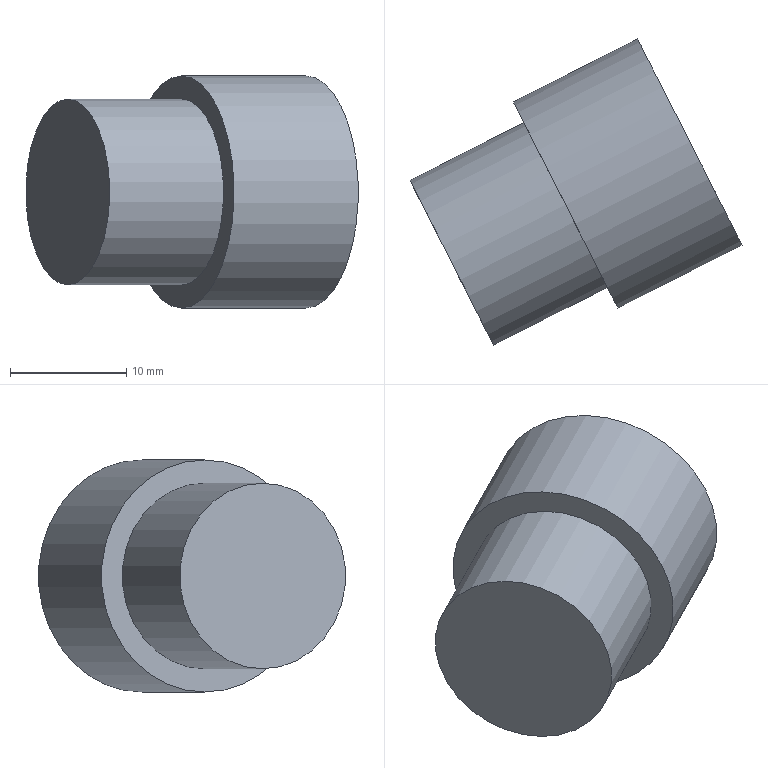Part | STEP file | solid 196 | 1 solid | 8 faces | box 28.652 x 26.452 x 20 mm | volume 5174 mm3 | cylinder 3 | plane 3 | cone 2 | commonest cylinder face diameters 8 x1 16 x1 20 x1